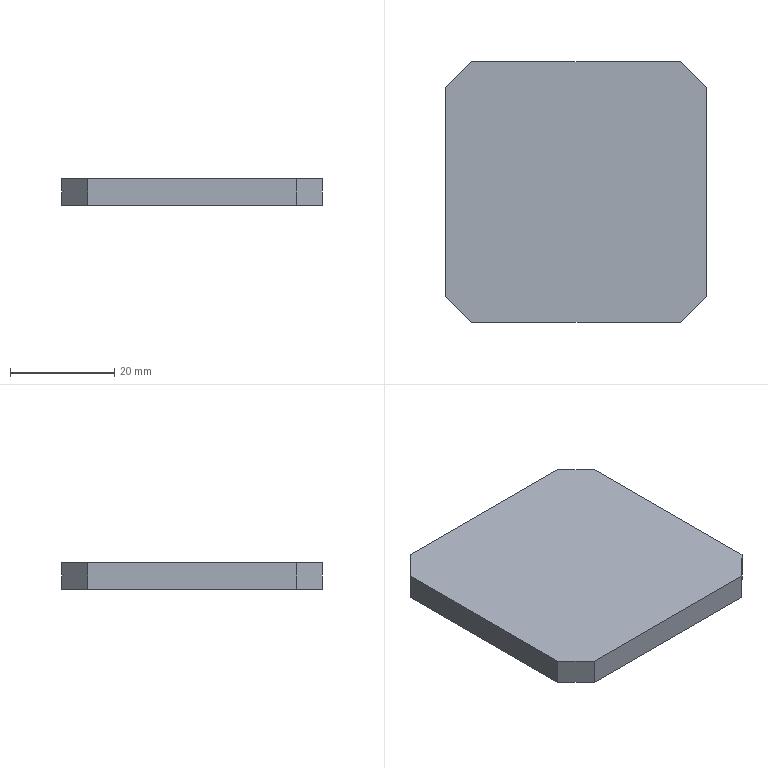Part | SolidWorks | features Chamfer 1, Extrusion 1 | 1 solid | 10 faces | box 50 x 50 x 5 mm | volume 12250 mm3 | plane 10
STEP:
#1=CARTESIAN_POINT('',(-24.459,23.42,0.));
#2=VERTEX_POINT('',#1);
#3=CARTESIAN_POINT('',(-24.459,-16.58,0.));
#4=VERTEX_POINT('',#3);
#5=CARTESIAN_POINT('',(-24.459,28.42,0.));
#6=DIRECTION('',(0.,-1.,0.));
#7=VECTOR('',#6,1000.);
#8=LINE('',#5,#7);
#9=EDGE_CURVE('',#2,#4,#8,.T.);
#10=ORIENTED_EDGE('',*,*,#9,.T.);
#11=CARTESIAN_POINT('',(-24.459,-16.58,5.));
#12=VERTEX_POINT('',#11);
#13=CARTESIAN_POINT('',(-24.459,-16.58,5.));
#14=DIRECTION('',(0.,0.,1.));
#15=VECTOR('',#14,1000.);
#16=LINE('',#13,#15);
#17=EDGE_CURVE('',#4,#12,#16,.T.);
#18=ORIENTED_EDGE('',*,*,#17,.T.);
#19=CARTESIAN_POINT('',(-24.459,23.42,5.));
#20=VERTEX_POINT('',#19);
#21=CARTESIAN_POINT('',(-24.459,28.42,5.));
#22=DIRECTION('',(0.,-1.,0.));
#23=VECTOR('',#22,1000.);
#24=LINE('',#21,#23);
#25=EDGE_CURVE('',#20,#12,#24,.T.);
#26=ORIENTED_EDGE('',*,*,#25,.F.);
#27=CARTESIAN_POINT('',(-24.459,23.42,5.));
#28=DIRECTION('',(0.,0.,-1.));
#29=VECTOR('',#28,1000.);
#30=LINE('',#27,#29);
#31=EDGE_CURVE('',#20,#2,#30,.T.);
#32=ORIENTED_EDGE('',*,*,#31,.T.);
#33=EDGE_LOOP('',(#10,#18,#26,#32));
#34=FACE_OUTER_BOUND('',#33,.T.);
#35=CARTESIAN_POINT('',(-24.459,28.42,5.));
#36=DIRECTION('',(1.,0.,0.));
#37=DIRECTION('',(0.,1.,0.));
#38=AXIS2_PLACEMENT_3D('',#35,#36,#37);
#39=PLANE('',#38);
#40=ADVANCED_FACE('',(#34),#39,.F.);
#41=CARTESIAN_POINT('',(-19.459,-21.58,5.));
#42=VERTEX_POINT('',#41);
#43=CARTESIAN_POINT('',(20.541,-21.58,5.));
#44=VERTEX_POINT('',#43);
#45=CARTESIAN_POINT('',(-24.459,-21.58,5.));
#46=DIRECTION('',(1.,0.,0.));
#47=VECTOR('',#46,1000.);
#48=LINE('',#45,#47);
#49=EDGE_CURVE('',#42,#44,#48,.T.);
#50=ORIENTED_EDGE('',*,*,#49,.F.);
#51=CARTESIAN_POINT('',(-19.459,-21.58,0.));
#52=VERTEX_POINT('',#51);
#53=CARTESIAN_POINT('',(-19.459,-21.58,5.));
#54=DIRECTION('',(0.,0.,-1.));
#55=VECTOR('',#54,1000.);
#56=LINE('',#53,#55);
#57=EDGE_CURVE('',#42,#52,#56,.T.);
#58=ORIENTED_EDGE('',*,*,#57,.T.);
#59=CARTESIAN_POINT('',(20.541,-21.58,0.));
#60=VERTEX_POINT('',#59);
#61=CARTESIAN_POINT('',(-24.459,-21.58,0.));
#62=DIRECTION('',(1.,0.,0.));
#63=VECTOR('',#62,1000.);
#64=LINE('',#61,#63);
#65=EDGE_CURVE('',#52,#60,#64,.T.);
#66=ORIENTED_EDGE('',*,*,#65,.T.);
#67=CARTESIAN_POINT('',(20.541,-21.58,5.));
#68=DIRECTION('',(0.,0.,1.));
#69=VECTOR('',#68,1000.);
#70=LINE('',#67,#69);
#71=EDGE_CURVE('',#60,#44,#70,.T.);
#72=ORIENTED_EDGE('',*,*,#71,.T.);
#73=EDGE_LOOP('',(#50,#58,#66,#72));
#74=FACE_OUTER_BOUND('',#73,.T.);
#75=CARTESIAN_POINT('',(-24.459,-21.58,5.));
#76=DIRECTION('',(0.,1.,0.));
#77=DIRECTION('',(0.,0.,1.));
#78=AXIS2_PLACEMENT_3D('',#75,#76,#77);
#79=PLANE('',#78);
#80=ADVANCED_FACE('',(#74),#79,.F.);
#81=CARTESIAN_POINT('',(25.541,-16.58,5.));
#82=VERTEX_POINT('',#81);
#83=CARTESIAN_POINT('',(25.541,23.42,5.));
#84=VERTEX_POINT('',#83);
#85=CARTESIAN_POINT('',(25.541,28.42,5.));
#86=DIRECTION('',(0.,1.,0.));
#87=VECTOR('',#86,1000.);
#88=LINE('',#85,#87);
#89=EDGE_CURVE('',#82,#84,#88,.T.);
#90=ORIENTED_EDGE('',*,*,#89,.F.);
#91=CARTESIAN_POINT('',(25.541,-16.58,0.));
#92=VERTEX_POINT('',#91);
#93=CARTESIAN_POINT('',(25.541,-16.58,5.));
#94=DIRECTION('',(0.,0.,-1.));
#95=VECTOR('',#94,1000.);
#96=LINE('',#93,#95);
#97=EDGE_CURVE('',#82,#92,#96,.T.);
#98=ORIENTED_EDGE('',*,*,#97,.T.);
#99=CARTESIAN_POINT('',(25.541,23.42,0.));
#100=VERTEX_POINT('',#99);
#101=CARTESIAN_POINT('',(25.541,28.42,0.));
#102=DIRECTION('',(0.,1.,0.));
#103=VECTOR('',#102,1000.);
#104=LINE('',#101,#103);
#105=EDGE_CURVE('',#92,#100,#104,.T.);
#106=ORIENTED_EDGE('',*,*,#105,.T.);
#107=CARTESIAN_POINT('',(25.541,23.42,5.));
#108=DIRECTION('',(0.,0.,1.));
#109=VECTOR('',#108,1000.);
#110=LINE('',#107,#109);
#111=EDGE_CURVE('',#100,#84,#110,.T.);
#112=ORIENTED_EDGE('',*,*,#111,.T.);
#113=EDGE_LOOP('',(#90,#98,#106,#112));
#114=FACE_OUTER_BOUND('',#113,.T.);
#115=CARTESIAN_POINT('',(25.541,28.42,5.));
#116=DIRECTION('',(-1.,0.,0.));
#117=DIRECTION('',(0.,-1.,0.));
#118=AXIS2_PLACEMENT_3D('',#115,#116,#117);
#119=PLANE('',#118);
#120=ADVANCED_FACE('',(#114),#119,.F.);
#121=CARTESIAN_POINT('',(20.541,28.42,5.));
#122=VERTEX_POINT('',#121);
#123=CARTESIAN_POINT('',(-19.459,28.42,5.));
#124=VERTEX_POINT('',#123);
#125=CARTESIAN_POINT('',(-24.459,28.42,5.));
#126=DIRECTION('',(-1.,0.,0.));
#127=VECTOR('',#126,1000.);
#128=LINE('',#125,#127);
#129=EDGE_CURVE('',#122,#124,#128,.T.);
#130=ORIENTED_EDGE('',*,*,#129,.F.);
#131=CARTESIAN_POINT('',(20.541,28.42,0.));
#132=VERTEX_POINT('',#131);
#133=CARTESIAN_POINT('',(20.541,28.42,5.));
#134=DIRECTION('',(0.,0.,-1.));
#135=VECTOR('',#134,1000.);
#136=LINE('',#133,#135);
#137=EDGE_CURVE('',#122,#132,#136,.T.);
#138=ORIENTED_EDGE('',*,*,#137,.T.);
#139=CARTESIAN_POINT('',(-19.459,28.42,0.));
#140=VERTEX_POINT('',#139);
#141=CARTESIAN_POINT('',(-24.459,28.42,0.));
#142=DIRECTION('',(-1.,0.,0.));
#143=VECTOR('',#142,1000.);
#144=LINE('',#141,#143);
#145=EDGE_CURVE('',#132,#140,#144,.T.);
#146=ORIENTED_EDGE('',*,*,#145,.T.);
#147=CARTESIAN_POINT('',(-19.459,28.42,5.));
#148=DIRECTION('',(0.,0.,1.));
#149=VECTOR('',#148,1000.);
#150=LINE('',#147,#149);
#151=EDGE_CURVE('',#140,#124,#150,.T.);
#152=ORIENTED_EDGE('',*,*,#151,.T.);
#153=EDGE_LOOP('',(#130,#138,#146,#152));
#154=FACE_OUTER_BOUND('',#153,.T.);
#155=CARTESIAN_POINT('',(-24.459,28.42,5.));
#156=DIRECTION('',(0.,-1.,0.));
#157=DIRECTION('',(0.,0.,-1.));
#158=AXIS2_PLACEMENT_3D('',#155,#156,#157);
#159=PLANE('',#158);
#160=ADVANCED_FACE('',(#154),#159,.F.);
#161=ORIENTED_EDGE('',*,*,#25,.T.);
#162=CARTESIAN_POINT('',(-20.52,-20.52,5.));
#163=DIRECTION('',(0.7071,-0.7071,0.));
#164=VECTOR('',#163,1000.);
#165=LINE('',#162,#164);
#166=EDGE_CURVE('',#12,#42,#165,.T.);
#167=ORIENTED_EDGE('',*,*,#166,.T.);
#168=ORIENTED_EDGE('',*,*,#49,.T.);
#169=CARTESIAN_POINT('',(21.061,-21.061,5.));
#170=DIRECTION('',(0.7071,0.7071,0.));
#171=VECTOR('',#170,1000.);
#172=LINE('',#169,#171);
#173=EDGE_CURVE('',#44,#82,#172,.T.);
#174=ORIENTED_EDGE('',*,*,#173,.T.);
#175=ORIENTED_EDGE('',*,*,#89,.T.);
#176=CARTESIAN_POINT('',(24.48,24.48,5.));
#177=DIRECTION('',(-0.7071,0.7071,0.));
#178=VECTOR('',#177,1000.);
#179=LINE('',#176,#178);
#180=EDGE_CURVE('',#84,#122,#179,.T.);
#181=ORIENTED_EDGE('',*,*,#180,.T.);
#182=ORIENTED_EDGE('',*,*,#129,.T.);
#183=CARTESIAN_POINT('',(-23.939,23.939,5.));
#184=DIRECTION('',(-0.7071,-0.7071,0.));
#185=VECTOR('',#184,1000.);
#186=LINE('',#183,#185);
#187=EDGE_CURVE('',#124,#20,#186,.T.);
#188=ORIENTED_EDGE('',*,*,#187,.T.);
#189=EDGE_LOOP('',(#161,#167,#168,#174,#175,#181,#182,#188));
#190=FACE_OUTER_BOUND('',#189,.T.);
#191=CARTESIAN_POINT('',(0.,0.,5.));
#192=DIRECTION('',(0.,0.,1.));
#193=DIRECTION('',(1.,0.,0.));
#194=AXIS2_PLACEMENT_3D('',#191,#192,#193);
#195=PLANE('',#194);
#196=ADVANCED_FACE('',(#190),#195,.T.);
#197=ORIENTED_EDGE('',*,*,#65,.F.);
#198=CARTESIAN_POINT('',(-19.459,-21.58,0.));
#199=DIRECTION('',(-0.7071,0.7071,0.));
#200=VECTOR('',#199,1000.);
#201=LINE('',#198,#200);
#202=EDGE_CURVE('',#52,#4,#201,.T.);
#203=ORIENTED_EDGE('',*,*,#202,.T.);
#204=ORIENTED_EDGE('',*,*,#9,.F.);
#205=CARTESIAN_POINT('',(-24.459,23.42,0.));
#206=DIRECTION('',(0.7071,0.7071,0.));
#207=VECTOR('',#206,1000.);
#208=LINE('',#205,#207);
#209=EDGE_CURVE('',#2,#140,#208,.T.);
#210=ORIENTED_EDGE('',*,*,#209,.T.);
#211=ORIENTED_EDGE('',*,*,#145,.F.);
#212=CARTESIAN_POINT('',(20.541,28.42,0.));
#213=DIRECTION('',(0.7071,-0.7071,0.));
#214=VECTOR('',#213,1000.);
#215=LINE('',#212,#214);
#216=EDGE_CURVE('',#132,#100,#215,.T.);
#217=ORIENTED_EDGE('',*,*,#216,.T.);
#218=ORIENTED_EDGE('',*,*,#105,.F.);
#219=CARTESIAN_POINT('',(25.541,-16.58,0.));
#220=DIRECTION('',(-0.7071,-0.7071,0.));
#221=VECTOR('',#220,1000.);
#222=LINE('',#219,#221);
#223=EDGE_CURVE('',#92,#60,#222,.T.);
#224=ORIENTED_EDGE('',*,*,#223,.T.);
#225=EDGE_LOOP('',(#197,#203,#204,#210,#211,#217,#218,#224));
#226=FACE_OUTER_BOUND('',#225,.T.);
#227=CARTESIAN_POINT('',(0.,0.,0.));
#228=DIRECTION('',(0.,0.,1.));
#229=DIRECTION('',(1.,0.,0.));
#230=AXIS2_PLACEMENT_3D('',#227,#228,#229);
#231=PLANE('',#230);
#232=ADVANCED_FACE('',(#226),#231,.F.);
#233=ORIENTED_EDGE('',*,*,#166,.F.);
#234=ORIENTED_EDGE('',*,*,#17,.F.);
#235=ORIENTED_EDGE('',*,*,#202,.F.);
#236=ORIENTED_EDGE('',*,*,#57,.F.);
#237=EDGE_LOOP('',(#233,#234,#235,#236));
#238=FACE_OUTER_BOUND('',#237,.T.);
#239=CARTESIAN_POINT('',(-19.459,-21.58,5.));
#240=DIRECTION('',(0.7071,0.7071,0.));
#241=DIRECTION('',(0.,0.,-1.));
#242=AXIS2_PLACEMENT_3D('',#239,#240,#241);
#243=PLANE('',#242);
#244=ADVANCED_FACE('',(#238),#243,.F.);
#245=ORIENTED_EDGE('',*,*,#173,.F.);
#246=ORIENTED_EDGE('',*,*,#71,.F.);
#247=ORIENTED_EDGE('',*,*,#223,.F.);
#248=ORIENTED_EDGE('',*,*,#97,.F.);
#249=EDGE_LOOP('',(#245,#246,#247,#248));
#250=FACE_OUTER_BOUND('',#249,.T.);
#251=CARTESIAN_POINT('',(25.541,-16.58,5.));
#252=DIRECTION('',(-0.7071,0.7071,0.));
#253=DIRECTION('',(0.,0.,-1.));
#254=AXIS2_PLACEMENT_3D('',#251,#252,#253);
#255=PLANE('',#254);
#256=ADVANCED_FACE('',(#250),#255,.F.);
#257=ORIENTED_EDGE('',*,*,#180,.F.);
#258=ORIENTED_EDGE('',*,*,#111,.F.);
#259=ORIENTED_EDGE('',*,*,#216,.F.);
#260=ORIENTED_EDGE('',*,*,#137,.F.);
#261=EDGE_LOOP('',(#257,#258,#259,#260));
#262=FACE_OUTER_BOUND('',#261,.T.);
#263=CARTESIAN_POINT('',(20.541,28.42,5.));
#264=DIRECTION('',(-0.7071,-0.7071,0.));
#265=DIRECTION('',(0.,0.,-1.));
#266=AXIS2_PLACEMENT_3D('',#263,#264,#265);
#267=PLANE('',#266);
#268=ADVANCED_FACE('',(#262),#267,.F.);
#269=ORIENTED_EDGE('',*,*,#187,.F.);
#270=ORIENTED_EDGE('',*,*,#151,.F.);
#271=ORIENTED_EDGE('',*,*,#209,.F.);
#272=ORIENTED_EDGE('',*,*,#31,.F.);
#273=EDGE_LOOP('',(#269,#270,#271,#272));
#274=FACE_OUTER_BOUND('',#273,.T.);
#275=CARTESIAN_POINT('',(-24.459,23.42,5.));
#276=DIRECTION('',(0.7071,-0.7071,0.));
#277=DIRECTION('',(0.,0.,-1.));
#278=AXIS2_PLACEMENT_3D('',#275,#276,#277);
#279=PLANE('',#278);
#280=ADVANCED_FACE('',(#274),#279,.F.);
#281=CLOSED_SHELL('',(#40,#80,#120,#160,#196,#232,#244,#256,#268,#280));
#282=MANIFOLD_SOLID_BREP('',#281);
#283=CARTESIAN_POINT('',(0.,0.,0.));
#284=DIRECTION('',(0.,0.,1.));
#285=DIRECTION('',(1.,0.,0.));
#286=AXIS2_PLACEMENT_3D('',#283,#284,#285);
#287=(LENGTH_UNIT()NAMED_UNIT(*)SI_UNIT(.MILLI.,.METRE.));
#288=UNCERTAINTY_MEASURE_WITH_UNIT(LENGTH_MEASURE(0.00001),#287,'','');
#289=(NAMED_UNIT(*)PLANE_ANGLE_UNIT()SI_UNIT($,.RADIAN.));
#290=(NAMED_UNIT(*)SI_UNIT($,.STERADIAN.)SOLID_ANGLE_UNIT());
#291=(GEOMETRIC_REPRESENTATION_CONTEXT(3)GLOBAL_UNCERTAINTY_ASSIGNED_CONTEXT((#288))GLOBAL_UNIT_ASSIGNED_CONTEXT((#287,#289,#290))REPRESENTATION_CONTEXT('',''));
#292=ADVANCED_BREP_SHAPE_REPRESENTATION('',(#282,#286),#291);